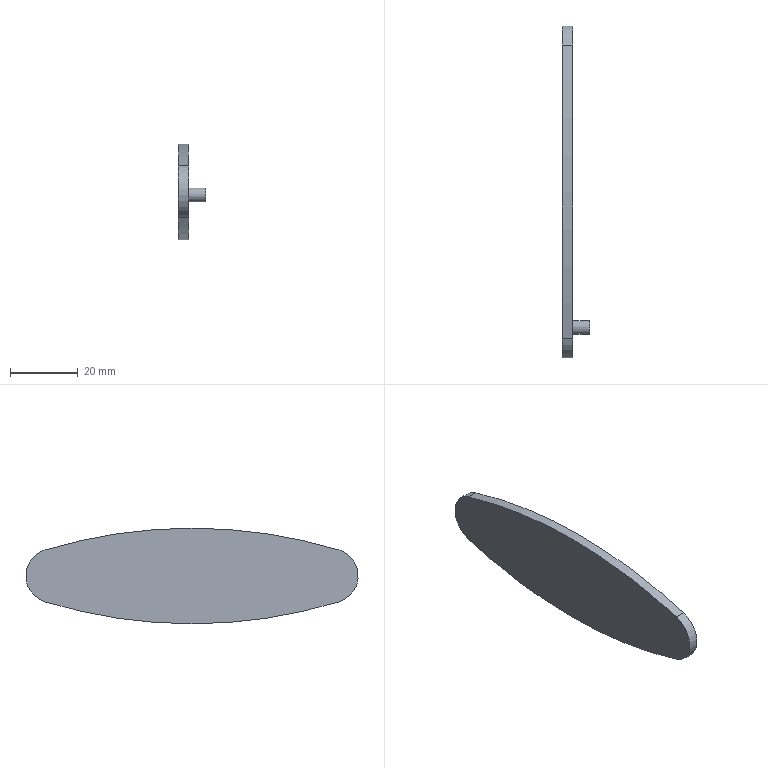Part | STEP file | zheyetulun | 1 solid | 8 faces | box 8 x 98.136 x 28.217 mm | volume 6682 mm3 | cylinder 5 | plane 3 | commonest cylinder face diameters 16 x2 4 x1 296.435 x1 300 x1
STEP:
#1=CARTESIAN_POINT('',(0.,0.,0.));
#2=DIRECTION('',(0.,0.,1.));
#3=DIRECTION('',(1.,0.,0.));
#4=AXIS2_PLACEMENT_3D('',#1,#2,#3);
#5=CARTESIAN_POINT('',(-1.5,-43.382,8.59));
#6=VERTEX_POINT('',#5);
#7=CARTESIAN_POINT('',(-1.5,-43.411,-6.718));
#8=VERTEX_POINT('',#7);
#9=CARTESIAN_POINT('',(-1.5,-41.068,0.9316));
#10=DIRECTION('',(1.,0.,0.));
#11=DIRECTION('',(0.,0.,-1.));
#12=AXIS2_PLACEMENT_3D('',#9,#10,#11);
#13=CIRCLE('',#12,8.);
#14=CARTESIAN_POINT('',(1.5,-41.068,0.9316));
#15=DIRECTION('',(-1.,0.,0.));
#16=DIRECTION('',(0.,0.,1.));
#17=AXIS2_PLACEMENT_3D('',#14,#15,#16);
#18=CYLINDRICAL_SURFACE('',#17,8.);
#19=CARTESIAN_POINT('',(9.425,3.));
#20=DIRECTION('',(-1.,0.));
#21=VECTOR('',#20,1.);
#22=LINE('',#19,#21);
#23=(GEOMETRIC_REPRESENTATION_CONTEXT(2)PARAMETRIC_REPRESENTATION_CONTEXT()REPRESENTATION_CONTEXT('',''));
#24=DEFINITIONAL_REPRESENTATION('',(#22),#23);
#25=PCURVE('',#18,#24);
#26=CARTESIAN_POINT('',(-1.5,-20.534,67.966));
#27=DIRECTION('',(1.,0.,0.));
#28=DIRECTION('',(0.,0.,-1.));
#29=AXIS2_PLACEMENT_3D('',#26,#27,#28);
#30=PLANE('',#29);
#31=CARTESIAN_POINT('',(67.034,-20.534));
#32=DIRECTION('',(1.,0.));
#33=AXIS2_PLACEMENT_2D('',#31,#32);
#34=CIRCLE('',#33,8.);
#35=(GEOMETRIC_REPRESENTATION_CONTEXT(2)PARAMETRIC_REPRESENTATION_CONTEXT()REPRESENTATION_CONTEXT('',''));
#36=DEFINITIONAL_REPRESENTATION('',(#34),#35);
#37=PCURVE('',#30,#36);
#38=SURFACE_CURVE('',#13,(#25,#37),.PCURVE_S1.);
#39=EDGE_CURVE('',#6,#8,#38,.T.);
#40=ORIENTED_EDGE('',*,*,#39,.T.);
#41=CARTESIAN_POINT('',(1.5,-43.411,-6.718));
#42=VERTEX_POINT('',#41);
#43=CARTESIAN_POINT('',(1.5,-43.411,-6.718));
#44=DIRECTION('',(-1.,0.,0.));
#45=VECTOR('',#44,1.);
#46=LINE('',#43,#45);
#47=CARTESIAN_POINT('',(3.439,0.));
#48=DIRECTION('',(0.,1.));
#49=VECTOR('',#48,1.);
#50=LINE('',#47,#49);
#51=(GEOMETRIC_REPRESENTATION_CONTEXT(2)PARAMETRIC_REPRESENTATION_CONTEXT()REPRESENTATION_CONTEXT('',''));
#52=DEFINITIONAL_REPRESENTATION('',(#50),#51);
#53=PCURVE('',#18,#52);
#54=CARTESIAN_POINT('',(1.5,0.,135.));
#55=DIRECTION('',(-1.,0.,0.));
#56=DIRECTION('',(0.,0.,1.));
#57=AXIS2_PLACEMENT_3D('',#54,#55,#56);
#58=CYLINDRICAL_SURFACE('',#57,148.217);
#59=CARTESIAN_POINT('',(3.439,0.));
#60=DIRECTION('',(0.,1.));
#61=VECTOR('',#60,1.);
#62=LINE('',#59,#61);
#63=(GEOMETRIC_REPRESENTATION_CONTEXT(2)PARAMETRIC_REPRESENTATION_CONTEXT()REPRESENTATION_CONTEXT('',''));
#64=DEFINITIONAL_REPRESENTATION('',(#62),#63);
#65=PCURVE('',#58,#64);
#66=SURFACE_CURVE('',#46,(#53,#65),.PCURVE_S1.);
#67=EDGE_CURVE('',#42,#8,#66,.T.);
#68=ORIENTED_EDGE('',*,*,#67,.F.);
#69=CARTESIAN_POINT('',(1.5,-43.382,8.59));
#70=VERTEX_POINT('',#69);
#71=CARTESIAN_POINT('',(1.5,-41.068,0.9316));
#72=DIRECTION('',(1.,0.,0.));
#73=DIRECTION('',(0.,0.,-1.));
#74=AXIS2_PLACEMENT_3D('',#71,#72,#73);
#75=CIRCLE('',#74,8.);
#76=CARTESIAN_POINT('',(9.425,0.));
#77=DIRECTION('',(-1.,0.));
#78=VECTOR('',#77,1.);
#79=LINE('',#76,#78);
#80=(GEOMETRIC_REPRESENTATION_CONTEXT(2)PARAMETRIC_REPRESENTATION_CONTEXT()REPRESENTATION_CONTEXT('',''));
#81=DEFINITIONAL_REPRESENTATION('',(#79),#80);
#82=PCURVE('',#18,#81);
#83=CARTESIAN_POINT('',(1.5,-20.534,67.966));
#84=DIRECTION('',(1.,0.,0.));
#85=DIRECTION('',(0.,0.,-1.));
#86=AXIS2_PLACEMENT_3D('',#83,#84,#85);
#87=PLANE('',#86);
#88=CARTESIAN_POINT('',(67.034,-20.534));
#89=DIRECTION('',(1.,0.));
#90=AXIS2_PLACEMENT_2D('',#88,#89);
#91=CIRCLE('',#90,8.);
#92=(GEOMETRIC_REPRESENTATION_CONTEXT(2)PARAMETRIC_REPRESENTATION_CONTEXT()REPRESENTATION_CONTEXT('',''));
#93=DEFINITIONAL_REPRESENTATION('',(#91),#92);
#94=PCURVE('',#87,#93);
#95=SURFACE_CURVE('',#75,(#82,#94),.PCURVE_S1.);
#96=EDGE_CURVE('',#70,#42,#95,.T.);
#97=ORIENTED_EDGE('',*,*,#96,.F.);
#98=CARTESIAN_POINT('',(1.5,-43.382,8.59));
#99=DIRECTION('',(-1.,0.,0.));
#100=VECTOR('',#99,1.);
#101=LINE('',#98,#100);
#102=CARTESIAN_POINT('',(5.99,0.));
#103=DIRECTION('',(0.,1.));
#104=VECTOR('',#103,1.);
#105=LINE('',#102,#104);
#106=(GEOMETRIC_REPRESENTATION_CONTEXT(2)PARAMETRIC_REPRESENTATION_CONTEXT()REPRESENTATION_CONTEXT('',''));
#107=DEFINITIONAL_REPRESENTATION('',(#105),#106);
#108=PCURVE('',#18,#107);
#109=CARTESIAN_POINT('',(1.5,0.,-135.));
#110=DIRECTION('',(-1.,0.,0.));
#111=DIRECTION('',(0.,0.,1.));
#112=AXIS2_PLACEMENT_3D('',#109,#110,#111);
#113=CYLINDRICAL_SURFACE('',#112,150.);
#114=CARTESIAN_POINT('',(-0.2934,0.));
#115=DIRECTION('',(0.,1.));
#116=VECTOR('',#115,1.);
#117=LINE('',#114,#116);
#118=(GEOMETRIC_REPRESENTATION_CONTEXT(2)PARAMETRIC_REPRESENTATION_CONTEXT()REPRESENTATION_CONTEXT('',''));
#119=DEFINITIONAL_REPRESENTATION('',(#117),#118);
#120=PCURVE('',#113,#119);
#121=SURFACE_CURVE('',#101,(#108,#120),.PCURVE_S1.);
#122=EDGE_CURVE('',#70,#6,#121,.T.);
#123=ORIENTED_EDGE('',*,*,#122,.T.);
#124=EDGE_LOOP('',(#40,#68,#97,#123));
#125=FACE_BOUND('',#124,.T.);
#126=ADVANCED_FACE('',(#125),#18,.T.);
#127=CARTESIAN_POINT('',(-1.5,43.411,-6.718));
#128=VERTEX_POINT('',#127);
#129=CARTESIAN_POINT('',(-1.5,0.,135.));
#130=DIRECTION('',(1.,0.,0.));
#131=DIRECTION('',(0.,0.,-1.));
#132=AXIS2_PLACEMENT_3D('',#129,#130,#131);
#133=CIRCLE('',#132,148.217);
#134=CARTESIAN_POINT('',(9.425,3.));
#135=DIRECTION('',(-1.,0.));
#136=VECTOR('',#135,1.);
#137=LINE('',#134,#136);
#138=(GEOMETRIC_REPRESENTATION_CONTEXT(2)PARAMETRIC_REPRESENTATION_CONTEXT()REPRESENTATION_CONTEXT('',''));
#139=DEFINITIONAL_REPRESENTATION('',(#137),#138);
#140=PCURVE('',#58,#139);
#141=CARTESIAN_POINT('',(-67.034,20.534));
#142=DIRECTION('',(1.,0.));
#143=AXIS2_PLACEMENT_2D('',#141,#142);
#144=CIRCLE('',#143,148.217);
#145=(GEOMETRIC_REPRESENTATION_CONTEXT(2)PARAMETRIC_REPRESENTATION_CONTEXT()REPRESENTATION_CONTEXT('',''));
#146=DEFINITIONAL_REPRESENTATION('',(#144),#145);
#147=PCURVE('',#30,#146);
#148=SURFACE_CURVE('',#133,(#140,#147),.PCURVE_S1.);
#149=EDGE_CURVE('',#8,#128,#148,.T.);
#150=ORIENTED_EDGE('',*,*,#149,.T.);
#151=CARTESIAN_POINT('',(1.5,43.411,-6.718));
#152=VERTEX_POINT('',#151);
#153=CARTESIAN_POINT('',(1.5,43.411,-6.718));
#154=DIRECTION('',(-1.,0.,0.));
#155=VECTOR('',#154,1.);
#156=LINE('',#153,#155);
#157=CARTESIAN_POINT('',(2.844,0.));
#158=DIRECTION('',(0.,1.));
#159=VECTOR('',#158,1.);
#160=LINE('',#157,#159);
#161=(GEOMETRIC_REPRESENTATION_CONTEXT(2)PARAMETRIC_REPRESENTATION_CONTEXT()REPRESENTATION_CONTEXT('',''));
#162=DEFINITIONAL_REPRESENTATION('',(#160),#161);
#163=PCURVE('',#58,#162);
#164=CARTESIAN_POINT('',(1.5,41.068,0.9316));
#165=DIRECTION('',(-1.,0.,0.));
#166=DIRECTION('',(0.,0.,1.));
#167=AXIS2_PLACEMENT_3D('',#164,#165,#166);
#168=CYLINDRICAL_SURFACE('',#167,8.);
#169=CARTESIAN_POINT('',(2.844,0.));
#170=DIRECTION('',(0.,1.));
#171=VECTOR('',#170,1.);
#172=LINE('',#169,#171);
#173=(GEOMETRIC_REPRESENTATION_CONTEXT(2)PARAMETRIC_REPRESENTATION_CONTEXT()REPRESENTATION_CONTEXT('',''));
#174=DEFINITIONAL_REPRESENTATION('',(#172),#173);
#175=PCURVE('',#168,#174);
#176=SURFACE_CURVE('',#156,(#163,#175),.PCURVE_S1.);
#177=EDGE_CURVE('',#152,#128,#176,.T.);
#178=ORIENTED_EDGE('',*,*,#177,.F.);
#179=CARTESIAN_POINT('',(1.5,0.,135.));
#180=DIRECTION('',(1.,0.,0.));
#181=DIRECTION('',(0.,0.,-1.));
#182=AXIS2_PLACEMENT_3D('',#179,#180,#181);
#183=CIRCLE('',#182,148.217);
#184=CARTESIAN_POINT('',(9.425,0.));
#185=DIRECTION('',(-1.,0.));
#186=VECTOR('',#185,1.);
#187=LINE('',#184,#186);
#188=(GEOMETRIC_REPRESENTATION_CONTEXT(2)PARAMETRIC_REPRESENTATION_CONTEXT()REPRESENTATION_CONTEXT('',''));
#189=DEFINITIONAL_REPRESENTATION('',(#187),#188);
#190=PCURVE('',#58,#189);
#191=CARTESIAN_POINT('',(-67.034,20.534));
#192=DIRECTION('',(1.,0.));
#193=AXIS2_PLACEMENT_2D('',#191,#192);
#194=CIRCLE('',#193,148.217);
#195=(GEOMETRIC_REPRESENTATION_CONTEXT(2)PARAMETRIC_REPRESENTATION_CONTEXT()REPRESENTATION_CONTEXT('',''));
#196=DEFINITIONAL_REPRESENTATION('',(#194),#195);
#197=PCURVE('',#87,#196);
#198=SURFACE_CURVE('',#183,(#190,#197),.PCURVE_S1.);
#199=EDGE_CURVE('',#42,#152,#198,.T.);
#200=ORIENTED_EDGE('',*,*,#199,.F.);
#201=ORIENTED_EDGE('',*,*,#67,.T.);
#202=EDGE_LOOP('',(#150,#178,#200,#201));
#203=FACE_BOUND('',#202,.T.);
#204=ADVANCED_FACE('',(#203),#58,.T.);
#205=CARTESIAN_POINT('',(-1.5,43.382,8.59));
#206=VERTEX_POINT('',#205);
#207=CARTESIAN_POINT('',(-1.5,41.068,0.9316));
#208=DIRECTION('',(1.,0.,0.));
#209=DIRECTION('',(0.,0.,1.));
#210=AXIS2_PLACEMENT_3D('',#207,#208,#209);
#211=CIRCLE('',#210,8.);
#212=CARTESIAN_POINT('',(6.283,3.));
#213=DIRECTION('',(-1.,0.));
#214=VECTOR('',#213,1.);
#215=LINE('',#212,#214);
#216=(GEOMETRIC_REPRESENTATION_CONTEXT(2)PARAMETRIC_REPRESENTATION_CONTEXT()REPRESENTATION_CONTEXT('',''));
#217=DEFINITIONAL_REPRESENTATION('',(#215),#216);
#218=PCURVE('',#168,#217);
#219=CARTESIAN_POINT('',(67.034,61.602));
#220=DIRECTION('',(-1.,0.));
#221=AXIS2_PLACEMENT_2D('',#219,#220);
#222=CIRCLE('',#221,8.);
#223=(GEOMETRIC_REPRESENTATION_CONTEXT(2)PARAMETRIC_REPRESENTATION_CONTEXT()REPRESENTATION_CONTEXT('',''));
#224=DEFINITIONAL_REPRESENTATION('',(#222),#223);
#225=PCURVE('',#30,#224);
#226=SURFACE_CURVE('',#211,(#218,#225),.PCURVE_S1.);
#227=EDGE_CURVE('',#128,#206,#226,.T.);
#228=ORIENTED_EDGE('',*,*,#227,.T.);
#229=CARTESIAN_POINT('',(1.5,43.382,8.59));
#230=VERTEX_POINT('',#229);
#231=CARTESIAN_POINT('',(1.5,43.382,8.59));
#232=DIRECTION('',(-1.,0.,0.));
#233=VECTOR('',#232,1.);
#234=LINE('',#231,#233);
#235=CARTESIAN_POINT('',(0.2934,0.));
#236=DIRECTION('',(0.,1.));
#237=VECTOR('',#236,1.);
#238=LINE('',#235,#237);
#239=(GEOMETRIC_REPRESENTATION_CONTEXT(2)PARAMETRIC_REPRESENTATION_CONTEXT()REPRESENTATION_CONTEXT('',''));
#240=DEFINITIONAL_REPRESENTATION('',(#238),#239);
#241=PCURVE('',#168,#240);
#242=CARTESIAN_POINT('',(0.2934,0.));
#243=DIRECTION('',(0.,1.));
#244=VECTOR('',#243,1.);
#245=LINE('',#242,#244);
#246=(GEOMETRIC_REPRESENTATION_CONTEXT(2)PARAMETRIC_REPRESENTATION_CONTEXT()REPRESENTATION_CONTEXT('',''));
#247=DEFINITIONAL_REPRESENTATION('',(#245),#246);
#248=PCURVE('',#113,#247);
#249=SURFACE_CURVE('',#234,(#241,#248),.PCURVE_S1.);
#250=EDGE_CURVE('',#230,#206,#249,.T.);
#251=ORIENTED_EDGE('',*,*,#250,.F.);
#252=CARTESIAN_POINT('',(1.5,41.068,0.9316));
#253=DIRECTION('',(1.,0.,0.));
#254=DIRECTION('',(0.,0.,1.));
#255=AXIS2_PLACEMENT_3D('',#252,#253,#254);
#256=CIRCLE('',#255,8.);
#257=CARTESIAN_POINT('',(6.283,0.));
#258=DIRECTION('',(-1.,0.));
#259=VECTOR('',#258,1.);
#260=LINE('',#257,#259);
#261=(GEOMETRIC_REPRESENTATION_CONTEXT(2)PARAMETRIC_REPRESENTATION_CONTEXT()REPRESENTATION_CONTEXT('',''));
#262=DEFINITIONAL_REPRESENTATION('',(#260),#261);
#263=PCURVE('',#168,#262);
#264=CARTESIAN_POINT('',(67.034,61.602));
#265=DIRECTION('',(-1.,0.));
#266=AXIS2_PLACEMENT_2D('',#264,#265);
#267=CIRCLE('',#266,8.);
#268=(GEOMETRIC_REPRESENTATION_CONTEXT(2)PARAMETRIC_REPRESENTATION_CONTEXT()REPRESENTATION_CONTEXT('',''));
#269=DEFINITIONAL_REPRESENTATION('',(#267),#268);
#270=PCURVE('',#87,#269);
#271=SURFACE_CURVE('',#256,(#263,#270),.PCURVE_S1.);
#272=EDGE_CURVE('',#152,#230,#271,.T.);
#273=ORIENTED_EDGE('',*,*,#272,.F.);
#274=ORIENTED_EDGE('',*,*,#177,.T.);
#275=EDGE_LOOP('',(#228,#251,#273,#274));
#276=FACE_BOUND('',#275,.T.);
#277=ADVANCED_FACE('',(#276),#168,.T.);
#278=CARTESIAN_POINT('',(-1.5,0.,-135.));
#279=DIRECTION('',(1.,0.,0.));
#280=DIRECTION('',(0.,0.,-1.));
#281=AXIS2_PLACEMENT_3D('',#278,#279,#280);
#282=CIRCLE('',#281,150.);
#283=CARTESIAN_POINT('',(3.142,3.));
#284=DIRECTION('',(-1.,0.));
#285=VECTOR('',#284,1.);
#286=LINE('',#283,#285);
#287=(GEOMETRIC_REPRESENTATION_CONTEXT(2)PARAMETRIC_REPRESENTATION_CONTEXT()REPRESENTATION_CONTEXT('',''));
#288=DEFINITIONAL_REPRESENTATION('',(#286),#287);
#289=PCURVE('',#113,#288);
#290=CARTESIAN_POINT('',(202.966,20.534));
#291=DIRECTION('',(1.,0.));
#292=AXIS2_PLACEMENT_2D('',#290,#291);
#293=CIRCLE('',#292,150.);
#294=(GEOMETRIC_REPRESENTATION_CONTEXT(2)PARAMETRIC_REPRESENTATION_CONTEXT()REPRESENTATION_CONTEXT('',''));
#295=DEFINITIONAL_REPRESENTATION('',(#293),#294);
#296=PCURVE('',#30,#295);
#297=SURFACE_CURVE('',#282,(#289,#296),.PCURVE_S1.);
#298=EDGE_CURVE('',#206,#6,#297,.T.);
#299=ORIENTED_EDGE('',*,*,#298,.T.);
#300=ORIENTED_EDGE('',*,*,#122,.F.);
#301=CARTESIAN_POINT('',(1.5,0.,-135.));
#302=DIRECTION('',(1.,0.,0.));
#303=DIRECTION('',(0.,0.,-1.));
#304=AXIS2_PLACEMENT_3D('',#301,#302,#303);
#305=CIRCLE('',#304,150.);
#306=CARTESIAN_POINT('',(3.142,0.));
#307=DIRECTION('',(-1.,0.));
#308=VECTOR('',#307,1.);
#309=LINE('',#306,#308);
#310=(GEOMETRIC_REPRESENTATION_CONTEXT(2)PARAMETRIC_REPRESENTATION_CONTEXT()REPRESENTATION_CONTEXT('',''));
#311=DEFINITIONAL_REPRESENTATION('',(#309),#310);
#312=PCURVE('',#113,#311);
#313=CARTESIAN_POINT('',(202.966,20.534));
#314=DIRECTION('',(1.,0.));
#315=AXIS2_PLACEMENT_2D('',#313,#314);
#316=CIRCLE('',#315,150.);
#317=(GEOMETRIC_REPRESENTATION_CONTEXT(2)PARAMETRIC_REPRESENTATION_CONTEXT()REPRESENTATION_CONTEXT('',''));
#318=DEFINITIONAL_REPRESENTATION('',(#316),#317);
#319=PCURVE('',#87,#318);
#320=SURFACE_CURVE('',#305,(#312,#319),.PCURVE_S1.);
#321=EDGE_CURVE('',#230,#70,#320,.T.);
#322=ORIENTED_EDGE('',*,*,#321,.F.);
#323=ORIENTED_EDGE('',*,*,#250,.T.);
#324=EDGE_LOOP('',(#299,#300,#322,#323));
#325=FACE_BOUND('',#324,.T.);
#326=ADVANCED_FACE('',(#325),#113,.T.);
#327=CARTESIAN_POINT('',(1.5,-40.,-2.));
#328=VERTEX_POINT('',#327);
#329=CARTESIAN_POINT('',(1.5,-40.,0.));
#330=DIRECTION('',(1.,0.,0.));
#331=DIRECTION('',(0.,0.,-1.));
#332=AXIS2_PLACEMENT_3D('',#329,#330,#331);
#333=CIRCLE('',#332,2.);
#334=CARTESIAN_POINT('',(67.966,-19.466));
#335=DIRECTION('',(1.,0.));
#336=AXIS2_PLACEMENT_2D('',#334,#335);
#337=CIRCLE('',#336,2.);
#338=(GEOMETRIC_REPRESENTATION_CONTEXT(2)PARAMETRIC_REPRESENTATION_CONTEXT()REPRESENTATION_CONTEXT('',''));
#339=DEFINITIONAL_REPRESENTATION('',(#337),#338);
#340=PCURVE('',#87,#339);
#341=CARTESIAN_POINT('',(6.5,-40.,0.));
#342=DIRECTION('',(-1.,0.,0.));
#343=DIRECTION('',(0.,0.,1.));
#344=AXIS2_PLACEMENT_3D('',#341,#342,#343);
#345=CYLINDRICAL_SURFACE('',#344,2.);
#346=CARTESIAN_POINT('',(9.425,5.));
#347=DIRECTION('',(-1.,0.));
#348=VECTOR('',#347,1.);
#349=LINE('',#346,#348);
#350=(GEOMETRIC_REPRESENTATION_CONTEXT(2)PARAMETRIC_REPRESENTATION_CONTEXT()REPRESENTATION_CONTEXT('',''));
#351=DEFINITIONAL_REPRESENTATION('',(#349),#350);
#352=PCURVE('',#345,#351);
#353=SURFACE_CURVE('',#333,(#340,#352),.PCURVE_S1.);
#354=EDGE_CURVE('',#328,#328,#353,.T.);
#355=ORIENTED_EDGE('',*,*,#354,.F.);
#356=EDGE_LOOP('',(#355));
#357=FACE_BOUND('',#356,.T.);
#358=ORIENTED_EDGE('',*,*,#96,.T.);
#359=ORIENTED_EDGE('',*,*,#199,.T.);
#360=ORIENTED_EDGE('',*,*,#272,.T.);
#361=ORIENTED_EDGE('',*,*,#321,.T.);
#362=EDGE_LOOP('',(#358,#359,#360,#361));
#363=FACE_BOUND('',#362,.T.);
#364=ADVANCED_FACE('',(#357,#363),#87,.T.);
#365=ORIENTED_EDGE('',*,*,#39,.F.);
#366=ORIENTED_EDGE('',*,*,#298,.F.);
#367=ORIENTED_EDGE('',*,*,#227,.F.);
#368=ORIENTED_EDGE('',*,*,#149,.F.);
#369=EDGE_LOOP('',(#365,#366,#367,#368));
#370=FACE_BOUND('',#369,.T.);
#371=ADVANCED_FACE('',(#370),#30,.F.);
#372=CARTESIAN_POINT('',(6.5,-40.,-2.));
#373=VERTEX_POINT('',#372);
#374=CARTESIAN_POINT('',(6.5,-40.,0.));
#375=DIRECTION('',(1.,0.,0.));
#376=DIRECTION('',(0.,0.,-1.));
#377=AXIS2_PLACEMENT_3D('',#374,#375,#376);
#378=CIRCLE('',#377,2.);
#379=CARTESIAN_POINT('',(9.425,0.));
#380=DIRECTION('',(-1.,0.));
#381=VECTOR('',#380,1.);
#382=LINE('',#379,#381);
#383=(GEOMETRIC_REPRESENTATION_CONTEXT(2)PARAMETRIC_REPRESENTATION_CONTEXT()REPRESENTATION_CONTEXT('',''));
#384=DEFINITIONAL_REPRESENTATION('',(#382),#383);
#385=PCURVE('',#345,#384);
#386=CARTESIAN_POINT('',(6.5,-40.,0.));
#387=DIRECTION('',(1.,0.,0.));
#388=DIRECTION('',(0.,0.,-1.));
#389=AXIS2_PLACEMENT_3D('',#386,#387,#388);
#390=PLANE('',#389);
#391=CARTESIAN_POINT('',(0.,0.));
#392=DIRECTION('',(1.,0.));
#393=AXIS2_PLACEMENT_2D('',#391,#392);
#394=CIRCLE('',#393,2.);
#395=(GEOMETRIC_REPRESENTATION_CONTEXT(2)PARAMETRIC_REPRESENTATION_CONTEXT()REPRESENTATION_CONTEXT('',''));
#396=DEFINITIONAL_REPRESENTATION('',(#394),#395);
#397=PCURVE('',#390,#396);
#398=SURFACE_CURVE('',#378,(#385,#397),.PCURVE_S1.);
#399=EDGE_CURVE('',#373,#373,#398,.T.);
#400=ORIENTED_EDGE('',*,*,#399,.F.);
#401=CARTESIAN_POINT('',(6.5,-40.,-2.));
#402=CARTESIAN_POINT('',(1.5,-40.,-2.));
#403=B_SPLINE_CURVE_WITH_KNOTS('',1,(#401,#402),.UNSPECIFIED.,.F.,.F.,(2,2),(0.,5.),.PIECEWISE_BEZIER_KNOTS.);
#404=CARTESIAN_POINT('',(9.425,0.));
#405=DIRECTION('',(0.,1.));
#406=VECTOR('',#405,1.);
#407=LINE('',#404,#406);
#408=(GEOMETRIC_REPRESENTATION_CONTEXT(2)PARAMETRIC_REPRESENTATION_CONTEXT()REPRESENTATION_CONTEXT('',''));
#409=DEFINITIONAL_REPRESENTATION('',(#407),#408);
#410=PCURVE('',#345,#409);
#411=CARTESIAN_POINT('',(3.142,0.));
#412=DIRECTION('',(0.,1.));
#413=VECTOR('',#412,1.);
#414=LINE('',#411,#413);
#415=(GEOMETRIC_REPRESENTATION_CONTEXT(2)PARAMETRIC_REPRESENTATION_CONTEXT()REPRESENTATION_CONTEXT('',''));
#416=DEFINITIONAL_REPRESENTATION('',(#414),#415);
#417=PCURVE('',#345,#416);
#418=SEAM_CURVE('',#403,(#410,#417),.PCURVE_S1.);
#419=EDGE_CURVE('',#373,#328,#418,.T.);
#420=ORIENTED_EDGE('',*,*,#419,.T.);
#421=ORIENTED_EDGE('',*,*,#354,.T.);
#422=ORIENTED_EDGE('',*,*,#419,.F.);
#423=EDGE_LOOP('',(#400,#420,#421,#422));
#424=FACE_BOUND('',#423,.T.);
#425=ADVANCED_FACE('',(#424),#345,.T.);
#426=ORIENTED_EDGE('',*,*,#399,.T.);
#427=EDGE_LOOP('',(#426));
#428=FACE_BOUND('',#427,.T.);
#429=ADVANCED_FACE('',(#428),#390,.T.);
#430=CLOSED_SHELL('',(#126,#204,#277,#326,#364,#371,#425,#429));
#431=MANIFOLD_SOLID_BREP('',#430);
#432=(LENGTH_UNIT()NAMED_UNIT(*)SI_UNIT(.MILLI.,.METRE.));
#433=UNCERTAINTY_MEASURE_WITH_UNIT(LENGTH_MEASURE(0.000002),#432,'','');
#434=(NAMED_UNIT(*)PLANE_ANGLE_UNIT()SI_UNIT($,.RADIAN.));
#435=(NAMED_UNIT(*)SI_UNIT($,.STERADIAN.)SOLID_ANGLE_UNIT());
#436=(GEOMETRIC_REPRESENTATION_CONTEXT(3)GLOBAL_UNCERTAINTY_ASSIGNED_CONTEXT((#433))GLOBAL_UNIT_ASSIGNED_CONTEXT((#432,#434,#435))REPRESENTATION_CONTEXT('',''));
#437=ADVANCED_BREP_SHAPE_REPRESENTATION('',(#4,#431),#436);